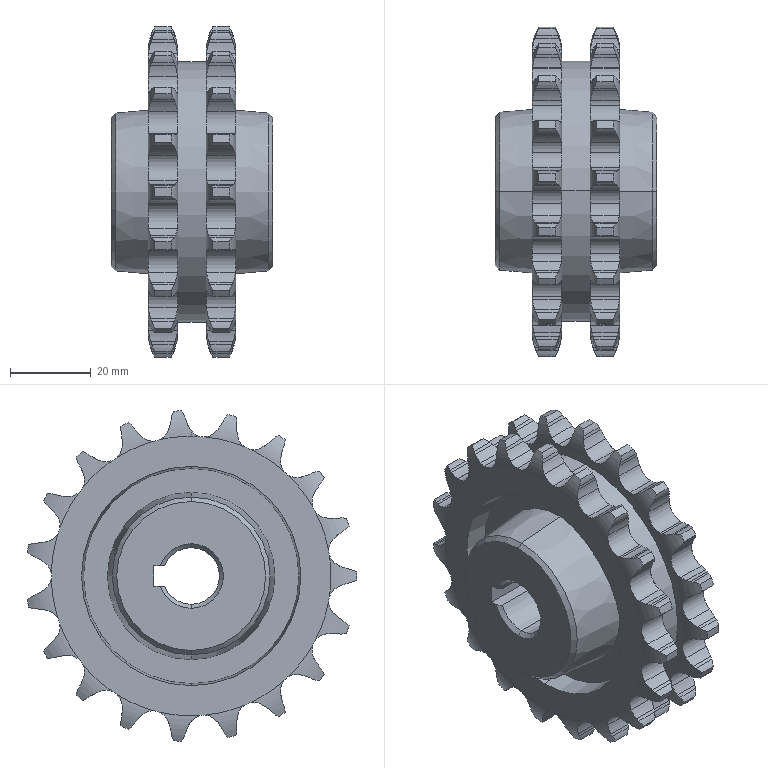Part | SolidWorks | features Cut 2, Revolution 2, Chamfer 1, CirPattern 1, LPattern 1 | 2 solids | 440 faces | box 40 x 81.595 x 81.862 mm | volume 93771 mm3 | cylinder 253 | plane 87 | torus 80 | cone 20 | commonest cylinder face diameters 11.518 x80 20.732 x80 8.06 x48 82 x38 14 x3 54.299 x2